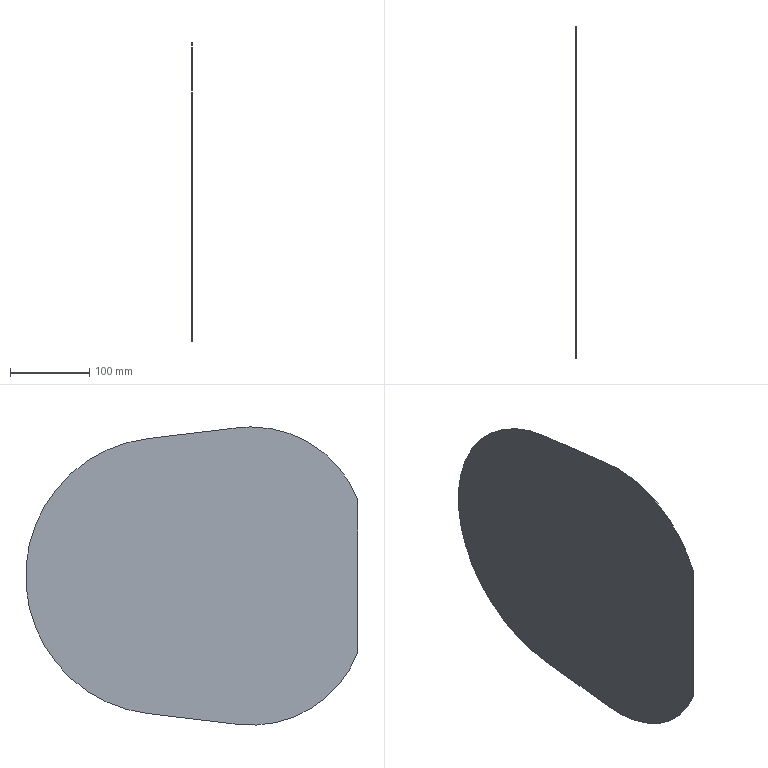Part | STEP file | Input 108 | 1 solid | 9 faces | box 0.5 x 420 x 377 mm | volume 66218 mm3 | plane 5 | cylinder 4 | commonest cylinder face diameters 288 x3 350 x1
STEP:
#1=CARTESIAN_POINT('',(0.,0.,0.));
#2=DIRECTION('',(0.,0.,1.));
#3=DIRECTION('',(1.,0.,0.));
#4=AXIS2_PLACEMENT_3D('',#1,#2,#3);
#5=CARTESIAN_POINT('',(3850.,420.,95.791));
#6=VERTEX_POINT('',#5);
#7=CARTESIAN_POINT('',(3850.,554.4,188.094));
#8=VERTEX_POINT('',#7);
#9=CARTESIAN_POINT('',(3850.,554.4,44.094));
#10=DIRECTION('',(-1.,0.,0.));
#11=DIRECTION('',(0.,0.,-1.));
#12=AXIS2_PLACEMENT_3D('',#9,#10,#11);
#13=CIRCLE('',#12,144.);
#14=CARTESIAN_POINT('',(4469.719,554.4,44.094));
#15=DIRECTION('',(-1.,0.,0.));
#16=DIRECTION('',(0.,0.,1.));
#17=AXIS2_PLACEMENT_3D('',#14,#15,#16);
#18=CYLINDRICAL_SURFACE('',#17,144.);
#19=CARTESIAN_POINT('',(3.142,619.719));
#20=DIRECTION('',(1.,0.));
#21=VECTOR('',#20,1.);
#22=LINE('',#19,#21);
#23=(GEOMETRIC_REPRESENTATION_CONTEXT(2)PARAMETRIC_REPRESENTATION_CONTEXT()REPRESENTATION_CONTEXT('',''));
#24=DEFINITIONAL_REPRESENTATION('',(#22),#23);
#25=PCURVE('',#18,#24);
#26=CARTESIAN_POINT('',(3850.,665.,-0.4063));
#27=DIRECTION('',(1.,0.,0.));
#28=DIRECTION('',(0.,0.,-1.));
#29=AXIS2_PLACEMENT_3D('',#26,#27,#28);
#30=PLANE('',#29);
#31=CARTESIAN_POINT('',(99.5,-110.6));
#32=CARTESIAN_POINT('',(99.5,-360.015));
#33=CARTESIAN_POINT('',(-116.5,-235.308));
#34=CARTESIAN_POINT('',(-332.5,-110.6));
#35=CARTESIAN_POINT('',(-116.5,14.108));
#36=CARTESIAN_POINT('',(99.5,138.815));
#37=CARTESIAN_POINT('',(99.5,-110.6));
#38=(BOUNDED_CURVE()B_SPLINE_CURVE(2,(#31,#32,#33,#34,#35,#36,#37),.UNSPECIFIED.,.T.,.F.)B_SPLINE_CURVE_WITH_KNOTS((1,2,2,2,2,1),(-2.094,0.,2.094,4.189,6.283,8.378),.UNSPECIFIED.)CURVE()GEOMETRIC_REPRESENTATION_ITEM()RATIONAL_B_SPLINE_CURVE((1.,0.5,1.,0.5,1.,0.5,1.))REPRESENTATION_ITEM(''));
#39=(GEOMETRIC_REPRESENTATION_CONTEXT(2)PARAMETRIC_REPRESENTATION_CONTEXT()REPRESENTATION_CONTEXT('',''));
#40=DEFINITIONAL_REPRESENTATION('',(#38),#39);
#41=PCURVE('',#30,#40);
#42=SURFACE_CURVE('',#13,(#25,#41),.PCURVE_S1.);
#43=EDGE_CURVE('',#6,#8,#42,.T.);
#44=ORIENTED_EDGE('',*,*,#43,.T.);
#45=CARTESIAN_POINT('',(3849.5,554.4,188.094));
#46=VERTEX_POINT('',#45);
#47=CARTESIAN_POINT('',(4469.719,554.4,188.094));
#48=DIRECTION('',(-1.,0.,0.));
#49=VECTOR('',#48,1.);
#50=LINE('',#47,#49);
#51=CARTESIAN_POINT('',(6.283,0.));
#52=DIRECTION('',(0.,1.));
#53=VECTOR('',#52,1.);
#54=LINE('',#51,#53);
#55=(GEOMETRIC_REPRESENTATION_CONTEXT(2)PARAMETRIC_REPRESENTATION_CONTEXT()REPRESENTATION_CONTEXT('',''));
#56=DEFINITIONAL_REPRESENTATION('',(#54),#55);
#57=PCURVE('',#18,#56);
#58=CARTESIAN_POINT('',(4469.719,554.4,44.094));
#59=DIRECTION('',(-1.,0.,0.));
#60=DIRECTION('',(0.,0.,1.));
#61=AXIS2_PLACEMENT_3D('',#58,#59,#60);
#62=CYLINDRICAL_SURFACE('',#61,144.);
#63=CARTESIAN_POINT('',(0.,0.));
#64=DIRECTION('',(0.,1.));
#65=VECTOR('',#64,1.);
#66=LINE('',#63,#65);
#67=(GEOMETRIC_REPRESENTATION_CONTEXT(2)PARAMETRIC_REPRESENTATION_CONTEXT()REPRESENTATION_CONTEXT('',''));
#68=DEFINITIONAL_REPRESENTATION('',(#66),#67);
#69=PCURVE('',#62,#68);
#70=SURFACE_CURVE('',#50,(#57,#69),.PCURVE_S1.);
#71=EDGE_CURVE('',#8,#46,#70,.T.);
#72=ORIENTED_EDGE('',*,*,#71,.T.);
#73=CARTESIAN_POINT('',(3849.5,420.,95.791));
#74=VERTEX_POINT('',#73);
#75=CARTESIAN_POINT('',(3849.5,554.4,44.094));
#76=DIRECTION('',(-1.,0.,0.));
#77=DIRECTION('',(0.,0.,1.));
#78=AXIS2_PLACEMENT_3D('',#75,#76,#77);
#79=CIRCLE('',#78,144.);
#80=CARTESIAN_POINT('',(0.,620.219));
#81=DIRECTION('',(1.,0.));
#82=VECTOR('',#81,1.);
#83=LINE('',#80,#82);
#84=(GEOMETRIC_REPRESENTATION_CONTEXT(2)PARAMETRIC_REPRESENTATION_CONTEXT()REPRESENTATION_CONTEXT('',''));
#85=DEFINITIONAL_REPRESENTATION('',(#83),#84);
#86=PCURVE('',#18,#85);
#87=CARTESIAN_POINT('',(3849.5,665.,-0.4063));
#88=DIRECTION('',(-1.,0.,0.));
#89=DIRECTION('',(0.,0.,1.));
#90=AXIS2_PLACEMENT_3D('',#87,#88,#89);
#91=PLANE('',#90);
#92=CARTESIAN_POINT('',(44.5,-110.6));
#93=DIRECTION('',(1.,0.));
#94=AXIS2_PLACEMENT_2D('',#92,#93);
#95=CIRCLE('',#94,144.);
#96=(GEOMETRIC_REPRESENTATION_CONTEXT(2)PARAMETRIC_REPRESENTATION_CONTEXT()REPRESENTATION_CONTEXT('',''));
#97=DEFINITIONAL_REPRESENTATION('',(#95),#96);
#98=PCURVE('',#91,#97);
#99=SURFACE_CURVE('',#79,(#86,#98),.PCURVE_S1.);
#100=EDGE_CURVE('',#74,#46,#99,.T.);
#101=ORIENTED_EDGE('',*,*,#100,.F.);
#102=CARTESIAN_POINT('',(4469.719,420.,95.791));
#103=DIRECTION('',(-1.,0.,0.));
#104=VECTOR('',#103,1.);
#105=LINE('',#102,#104);
#106=CARTESIAN_POINT('',(5.08,0.));
#107=DIRECTION('',(0.,1.));
#108=VECTOR('',#107,1.);
#109=LINE('',#106,#108);
#110=(GEOMETRIC_REPRESENTATION_CONTEXT(2)PARAMETRIC_REPRESENTATION_CONTEXT()REPRESENTATION_CONTEXT('',''));
#111=DEFINITIONAL_REPRESENTATION('',(#109),#110);
#112=PCURVE('',#18,#111);
#113=CARTESIAN_POINT('',(4469.719,420.,-96.604));
#114=DIRECTION('',(0.,-1.,0.));
#115=DIRECTION('',(0.,0.,1.));
#116=AXIS2_PLACEMENT_3D('',#113,#114,#115);
#117=PLANE('',#116);
#118=CARTESIAN_POINT('',(192.395,0.));
#119=DIRECTION('',(0.,1.));
#120=VECTOR('',#119,1.);
#121=LINE('',#118,#120);
#122=(GEOMETRIC_REPRESENTATION_CONTEXT(2)PARAMETRIC_REPRESENTATION_CONTEXT()REPRESENTATION_CONTEXT('',''));
#123=DEFINITIONAL_REPRESENTATION('',(#121),#122);
#124=PCURVE('',#117,#123);
#125=SURFACE_CURVE('',#105,(#112,#124),.PCURVE_S1.);
#126=EDGE_CURVE('',#6,#74,#125,.T.);
#127=ORIENTED_EDGE('',*,*,#126,.F.);
#128=EDGE_LOOP('',(#44,#72,#101,#127));
#129=FACE_BOUND('',#128,.T.);
#130=ADVANCED_FACE('',(#129),#18,.T.);
#131=CARTESIAN_POINT('',(3849.5,685.859,-174.159));
#132=VERTEX_POINT('',#131);
#133=CARTESIAN_POINT('',(3849.5,685.859,173.346));
#134=VERTEX_POINT('',#133);
#135=CARTESIAN_POINT('',(3849.5,665.,-0.4063));
#136=DIRECTION('',(1.,0.,0.));
#137=DIRECTION('',(0.,0.,-1.));
#138=AXIS2_PLACEMENT_3D('',#135,#136,#137);
#139=CIRCLE('',#138,175.);
#140=CARTESIAN_POINT('',(-175.,0.));
#141=CARTESIAN_POINT('',(-175.,303.109));
#142=CARTESIAN_POINT('',(87.5,151.554));
#143=CARTESIAN_POINT('',(350.,0.));
#144=CARTESIAN_POINT('',(87.5,-151.554));
#145=CARTESIAN_POINT('',(-175.,-303.109));
#146=CARTESIAN_POINT('',(-175.,0.));
#147=(BOUNDED_CURVE()B_SPLINE_CURVE(2,(#140,#141,#142,#143,#144,#145,#146),.UNSPECIFIED.,.T.,.F.)B_SPLINE_CURVE_WITH_KNOTS((1,2,2,2,2,1),(-2.094,0.,2.094,4.189,6.283,8.378),.UNSPECIFIED.)CURVE()GEOMETRIC_REPRESENTATION_ITEM()RATIONAL_B_SPLINE_CURVE((1.,0.5,1.,0.5,1.,0.5,1.))REPRESENTATION_ITEM(''));
#148=(GEOMETRIC_REPRESENTATION_CONTEXT(2)PARAMETRIC_REPRESENTATION_CONTEXT()REPRESENTATION_CONTEXT('',''));
#149=DEFINITIONAL_REPRESENTATION('',(#147),#148);
#150=PCURVE('',#91,#149);
#151=CARTESIAN_POINT('',(3850.,665.,-0.4063));
#152=DIRECTION('',(-1.,0.,0.));
#153=DIRECTION('',(0.,0.,1.));
#154=AXIS2_PLACEMENT_3D('',#151,#152,#153);
#155=CYLINDRICAL_SURFACE('',#154,175.);
#156=CARTESIAN_POINT('',(3.142,0.5));
#157=DIRECTION('',(-1.,0.));
#158=VECTOR('',#157,1.);
#159=LINE('',#156,#158);
#160=(GEOMETRIC_REPRESENTATION_CONTEXT(2)PARAMETRIC_REPRESENTATION_CONTEXT()REPRESENTATION_CONTEXT('',''));
#161=DEFINITIONAL_REPRESENTATION('',(#159),#160);
#162=PCURVE('',#155,#161);
#163=SURFACE_CURVE('',#139,(#150,#162),.PCURVE_S1.);
#164=EDGE_CURVE('',#132,#134,#163,.T.);
#165=ORIENTED_EDGE('',*,*,#164,.F.);
#166=CARTESIAN_POINT('',(3849.5,571.564,-187.88));
#167=VERTEX_POINT('',#166);
#168=CARTESIAN_POINT('',(3849.5,685.859,-174.159));
#169=DIRECTION('',(0.,-0.9929,-0.1192));
#170=VECTOR('',#169,1.);
#171=LINE('',#168,#170);
#172=CARTESIAN_POINT('',(-173.752,20.859));
#173=DIRECTION('',(-0.1192,-0.9929));
#174=VECTOR('',#173,1.);
#175=LINE('',#172,#174);
#176=(GEOMETRIC_REPRESENTATION_CONTEXT(2)PARAMETRIC_REPRESENTATION_CONTEXT()REPRESENTATION_CONTEXT('',''));
#177=DEFINITIONAL_REPRESENTATION('',(#175),#176);
#178=PCURVE('',#91,#177);
#179=CARTESIAN_POINT('',(4469.719,685.859,-174.159));
#180=DIRECTION('',(0.,0.1192,-0.9929));
#181=DIRECTION('',(0.,-0.9929,-0.1192));
#182=AXIS2_PLACEMENT_3D('',#179,#180,#181);
#183=PLANE('',#182);
#184=CARTESIAN_POINT('',(0.,620.219));
#185=DIRECTION('',(1.,0.));
#186=VECTOR('',#185,1.);
#187=LINE('',#184,#186);
#188=(GEOMETRIC_REPRESENTATION_CONTEXT(2)PARAMETRIC_REPRESENTATION_CONTEXT()REPRESENTATION_CONTEXT('',''));
#189=DEFINITIONAL_REPRESENTATION('',(#187),#188);
#190=PCURVE('',#183,#189);
#191=SURFACE_CURVE('',#171,(#178,#190),.PCURVE_S1.);
#192=EDGE_CURVE('',#132,#167,#191,.T.);
#193=ORIENTED_EDGE('',*,*,#192,.T.);
#194=CARTESIAN_POINT('',(3849.5,420.,-96.604));
#195=VERTEX_POINT('',#194);
#196=CARTESIAN_POINT('',(3849.5,554.4,-44.906));
#197=DIRECTION('',(-1.,0.,0.));
#198=DIRECTION('',(0.,0.,1.));
#199=AXIS2_PLACEMENT_3D('',#196,#197,#198);
#200=CIRCLE('',#199,144.);
#201=CARTESIAN_POINT('',(-44.5,-110.6));
#202=DIRECTION('',(1.,0.));
#203=AXIS2_PLACEMENT_2D('',#201,#202);
#204=CIRCLE('',#203,144.);
#205=(GEOMETRIC_REPRESENTATION_CONTEXT(2)PARAMETRIC_REPRESENTATION_CONTEXT()REPRESENTATION_CONTEXT('',''));
#206=DEFINITIONAL_REPRESENTATION('',(#204),#205);
#207=PCURVE('',#91,#206);
#208=CARTESIAN_POINT('',(4469.719,554.4,-44.906));
#209=DIRECTION('',(-1.,0.,0.));
#210=DIRECTION('',(0.,0.,1.));
#211=AXIS2_PLACEMENT_3D('',#208,#209,#210);
#212=CYLINDRICAL_SURFACE('',#211,144.);
#213=CARTESIAN_POINT('',(0.,620.219));
#214=DIRECTION('',(1.,0.));
#215=VECTOR('',#214,1.);
#216=LINE('',#213,#215);
#217=(GEOMETRIC_REPRESENTATION_CONTEXT(2)PARAMETRIC_REPRESENTATION_CONTEXT()REPRESENTATION_CONTEXT('',''));
#218=DEFINITIONAL_REPRESENTATION('',(#216),#217);
#219=PCURVE('',#212,#218);
#220=SURFACE_CURVE('',#200,(#207,#219),.PCURVE_S1.);
#221=EDGE_CURVE('',#167,#195,#220,.T.);
#222=ORIENTED_EDGE('',*,*,#221,.T.);
#223=CARTESIAN_POINT('',(3849.5,420.,-96.604));
#224=DIRECTION('',(0.,0.,1.));
#225=VECTOR('',#224,1.);
#226=LINE('',#223,#225);
#227=CARTESIAN_POINT('',(-96.198,-245.));
#228=DIRECTION('',(1.,0.));
#229=VECTOR('',#228,1.);
#230=LINE('',#227,#229);
#231=(GEOMETRIC_REPRESENTATION_CONTEXT(2)PARAMETRIC_REPRESENTATION_CONTEXT()REPRESENTATION_CONTEXT('',''));
#232=DEFINITIONAL_REPRESENTATION('',(#230),#231);
#233=PCURVE('',#91,#232);
#234=CARTESIAN_POINT('',(0.,620.219));
#235=DIRECTION('',(1.,0.));
#236=VECTOR('',#235,1.);
#237=LINE('',#234,#236);
#238=(GEOMETRIC_REPRESENTATION_CONTEXT(2)PARAMETRIC_REPRESENTATION_CONTEXT()REPRESENTATION_CONTEXT('',''));
#239=DEFINITIONAL_REPRESENTATION('',(#237),#238);
#240=PCURVE('',#117,#239);
#241=SURFACE_CURVE('',#226,(#233,#240),.PCURVE_S1.);
#242=EDGE_CURVE('',#195,#74,#241,.T.);
#243=ORIENTED_EDGE('',*,*,#242,.T.);
#244=ORIENTED_EDGE('',*,*,#100,.T.);
#245=CARTESIAN_POINT('',(3849.5,571.564,187.067));
#246=VERTEX_POINT('',#245);
#247=CARTESIAN_POINT('',(3849.5,554.4,44.094));
#248=DIRECTION('',(-1.,0.,0.));
#249=DIRECTION('',(0.,0.,1.));
#250=AXIS2_PLACEMENT_3D('',#247,#248,#249);
#251=CIRCLE('',#250,144.);
#252=CARTESIAN_POINT('',(44.5,-110.6));
#253=DIRECTION('',(1.,0.));
#254=AXIS2_PLACEMENT_2D('',#252,#253);
#255=CIRCLE('',#254,144.);
#256=(GEOMETRIC_REPRESENTATION_CONTEXT(2)PARAMETRIC_REPRESENTATION_CONTEXT()REPRESENTATION_CONTEXT('',''));
#257=DEFINITIONAL_REPRESENTATION('',(#255),#256);
#258=PCURVE('',#91,#257);
#259=CARTESIAN_POINT('',(0.,620.219));
#260=DIRECTION('',(1.,0.));
#261=VECTOR('',#260,1.);
#262=LINE('',#259,#261);
#263=(GEOMETRIC_REPRESENTATION_CONTEXT(2)PARAMETRIC_REPRESENTATION_CONTEXT()REPRESENTATION_CONTEXT('',''));
#264=DEFINITIONAL_REPRESENTATION('',(#262),#263);
#265=PCURVE('',#62,#264);
#266=SURFACE_CURVE('',#251,(#258,#265),.PCURVE_S1.);
#267=EDGE_CURVE('',#46,#246,#266,.T.);
#268=ORIENTED_EDGE('',*,*,#267,.T.);
#269=CARTESIAN_POINT('',(3849.5,571.564,187.067));
#270=DIRECTION('',(0.,0.9929,-0.1192));
#271=VECTOR('',#270,1.);
#272=LINE('',#269,#271);
#273=CARTESIAN_POINT('',(187.473,-93.436));
#274=DIRECTION('',(-0.1192,0.9929));
#275=VECTOR('',#274,1.);
#276=LINE('',#273,#275);
#277=(GEOMETRIC_REPRESENTATION_CONTEXT(2)PARAMETRIC_REPRESENTATION_CONTEXT()REPRESENTATION_CONTEXT('',''));
#278=DEFINITIONAL_REPRESENTATION('',(#276),#277);
#279=PCURVE('',#91,#278);
#280=CARTESIAN_POINT('',(4469.719,571.564,187.067));
#281=DIRECTION('',(0.,0.1192,0.9929));
#282=DIRECTION('',(0.,0.9929,-0.1192));
#283=AXIS2_PLACEMENT_3D('',#280,#281,#282);
#284=PLANE('',#283);
#285=CARTESIAN_POINT('',(0.,620.219));
#286=DIRECTION('',(1.,0.));
#287=VECTOR('',#286,1.);
#288=LINE('',#285,#287);
#289=(GEOMETRIC_REPRESENTATION_CONTEXT(2)PARAMETRIC_REPRESENTATION_CONTEXT()REPRESENTATION_CONTEXT('',''));
#290=DEFINITIONAL_REPRESENTATION('',(#288),#289);
#291=PCURVE('',#284,#290);
#292=SURFACE_CURVE('',#272,(#279,#291),.PCURVE_S1.);
#293=EDGE_CURVE('',#246,#134,#292,.T.);
#294=ORIENTED_EDGE('',*,*,#293,.T.);
#295=EDGE_LOOP('',(#165,#193,#222,#243,#244,#268,#294));
#296=FACE_BOUND('',#295,.T.);
#297=ADVANCED_FACE('',(#296),#91,.T.);
#298=CARTESIAN_POINT('',(3850.,685.859,173.346));
#299=VERTEX_POINT('',#298);
#300=CARTESIAN_POINT('',(3850.,685.859,-174.159));
#301=VERTEX_POINT('',#300);
#302=CARTESIAN_POINT('',(3850.,665.,-0.4063));
#303=DIRECTION('',(-1.,0.,0.));
#304=DIRECTION('',(0.,0.,1.));
#305=AXIS2_PLACEMENT_3D('',#302,#303,#304);
#306=CIRCLE('',#305,175.);
#307=CARTESIAN_POINT('',(-175.,0.));
#308=CARTESIAN_POINT('',(-175.,303.109));
#309=CARTESIAN_POINT('',(87.5,151.554));
#310=CARTESIAN_POINT('',(350.,0.));
#311=CARTESIAN_POINT('',(87.5,-151.554));
#312=CARTESIAN_POINT('',(-175.,-303.109));
#313=CARTESIAN_POINT('',(-175.,0.));
#314=(BOUNDED_CURVE()B_SPLINE_CURVE(2,(#307,#308,#309,#310,#311,#312,#313),.UNSPECIFIED.,.T.,.F.)B_SPLINE_CURVE_WITH_KNOTS((1,2,2,2,2,1),(-2.094,0.,2.094,4.189,6.283,8.378),.UNSPECIFIED.)CURVE()GEOMETRIC_REPRESENTATION_ITEM()RATIONAL_B_SPLINE_CURVE((1.,0.5,1.,0.5,1.,0.5,1.))REPRESENTATION_ITEM(''));
#315=(GEOMETRIC_REPRESENTATION_CONTEXT(2)PARAMETRIC_REPRESENTATION_CONTEXT()REPRESENTATION_CONTEXT('',''));
#316=DEFINITIONAL_REPRESENTATION('',(#314),#315);
#317=PCURVE('',#30,#316);
#318=CARTESIAN_POINT('',(0.,0.));
#319=DIRECTION('',(1.,0.));
#320=VECTOR('',#319,1.);
#321=LINE('',#318,#320);
#322=(GEOMETRIC_REPRESENTATION_CONTEXT(2)PARAMETRIC_REPRESENTATION_CONTEXT()REPRESENTATION_CONTEXT('',''));
#323=DEFINITIONAL_REPRESENTATION('',(#321),#322);
#324=PCURVE('',#155,#323);
#325=SURFACE_CURVE('',#306,(#317,#324),.PCURVE_S1.);
#326=EDGE_CURVE('',#299,#301,#325,.T.);
#327=ORIENTED_EDGE('',*,*,#326,.F.);
#328=CARTESIAN_POINT('',(3850.,571.564,187.067));
#329=VERTEX_POINT('',#328);
#330=CARTESIAN_POINT('',(3850.,571.564,187.067));
#331=DIRECTION('',(0.,0.9929,-0.1192));
#332=VECTOR('',#331,1.);
#333=LINE('',#330,#332);
#334=CARTESIAN_POINT('',(-187.473,-93.436));
#335=DIRECTION('',(0.1192,0.9929));
#336=VECTOR('',#335,1.);
#337=LINE('',#334,#336);
#338=(GEOMETRIC_REPRESENTATION_CONTEXT(2)PARAMETRIC_REPRESENTATION_CONTEXT()REPRESENTATION_CONTEXT('',''));
#339=DEFINITIONAL_REPRESENTATION('',(#337),#338);
#340=PCURVE('',#30,#339);
#341=CARTESIAN_POINT('',(0.,619.719));
#342=DIRECTION('',(1.,0.));
#343=VECTOR('',#342,1.);
#344=LINE('',#341,#343);
#345=(GEOMETRIC_REPRESENTATION_CONTEXT(2)PARAMETRIC_REPRESENTATION_CONTEXT()REPRESENTATION_CONTEXT('',''));
#346=DEFINITIONAL_REPRESENTATION('',(#344),#345);
#347=PCURVE('',#284,#346);
#348=SURFACE_CURVE('',#333,(#340,#347),.PCURVE_S1.);
#349=EDGE_CURVE('',#329,#299,#348,.T.);
#350=ORIENTED_EDGE('',*,*,#349,.F.);
#351=CARTESIAN_POINT('',(3850.,554.4,44.094));
#352=DIRECTION('',(-1.,0.,0.));
#353=DIRECTION('',(0.,0.,-1.));
#354=AXIS2_PLACEMENT_3D('',#351,#352,#353);
#355=CIRCLE('',#354,144.);
#356=CARTESIAN_POINT('',(99.5,-110.6));
#357=CARTESIAN_POINT('',(99.5,-360.015));
#358=CARTESIAN_POINT('',(-116.5,-235.308));
#359=CARTESIAN_POINT('',(-332.5,-110.6));
#360=CARTESIAN_POINT('',(-116.5,14.108));
#361=CARTESIAN_POINT('',(99.5,138.815));
#362=CARTESIAN_POINT('',(99.5,-110.6));
#363=(BOUNDED_CURVE()B_SPLINE_CURVE(2,(#356,#357,#358,#359,#360,#361,#362),.UNSPECIFIED.,.T.,.F.)B_SPLINE_CURVE_WITH_KNOTS((1,2,2,2,2,1),(-2.094,0.,2.094,4.189,6.283,8.378),.UNSPECIFIED.)CURVE()GEOMETRIC_REPRESENTATION_ITEM()RATIONAL_B_SPLINE_CURVE((1.,0.5,1.,0.5,1.,0.5,1.))REPRESENTATION_ITEM(''));
#364=(GEOMETRIC_REPRESENTATION_CONTEXT(2)PARAMETRIC_REPRESENTATION_CONTEXT()REPRESENTATION_CONTEXT('',''));
#365=DEFINITIONAL_REPRESENTATION('',(#363),#364);
#366=PCURVE('',#30,#365);
#367=CARTESIAN_POINT('',(-3.142,619.719));
#368=DIRECTION('',(1.,0.));
#369=VECTOR('',#368,1.);
#370=LINE('',#367,#369);
#371=(GEOMETRIC_REPRESENTATION_CONTEXT(2)PARAMETRIC_REPRESENTATION_CONTEXT()REPRESENTATION_CONTEXT('',''));
#372=DEFINITIONAL_REPRESENTATION('',(#370),#371);
#373=PCURVE('',#62,#372);
#374=SURFACE_CURVE('',#355,(#366,#373),.PCURVE_S1.);
#375=EDGE_CURVE('',#8,#329,#374,.T.);
#376=ORIENTED_EDGE('',*,*,#375,.F.);
#377=ORIENTED_EDGE('',*,*,#43,.F.);
#378=CARTESIAN_POINT('',(3850.,420.,-96.604));
#379=VERTEX_POINT('',#378);
#380=CARTESIAN_POINT('',(3850.,420.,-96.604));
#381=DIRECTION('',(0.,0.,1.));
#382=VECTOR('',#381,1.);
#383=LINE('',#380,#382);
#384=CARTESIAN_POINT('',(96.198,-245.));
#385=DIRECTION('',(-1.,0.));
#386=VECTOR('',#385,1.);
#387=LINE('',#384,#386);
#388=(GEOMETRIC_REPRESENTATION_CONTEXT(2)PARAMETRIC_REPRESENTATION_CONTEXT()REPRESENTATION_CONTEXT('',''));
#389=DEFINITIONAL_REPRESENTATION('',(#387),#388);
#390=PCURVE('',#30,#389);
#391=CARTESIAN_POINT('',(0.,619.719));
#392=DIRECTION('',(1.,0.));
#393=VECTOR('',#392,1.);
#394=LINE('',#391,#393);
#395=(GEOMETRIC_REPRESENTATION_CONTEXT(2)PARAMETRIC_REPRESENTATION_CONTEXT()REPRESENTATION_CONTEXT('',''));
#396=DEFINITIONAL_REPRESENTATION('',(#394),#395);
#397=PCURVE('',#117,#396);
#398=SURFACE_CURVE('',#383,(#390,#397),.PCURVE_S1.);
#399=EDGE_CURVE('',#379,#6,#398,.T.);
#400=ORIENTED_EDGE('',*,*,#399,.F.);
#401=CARTESIAN_POINT('',(3850.,571.564,-187.88));
#402=VERTEX_POINT('',#401);
#403=CARTESIAN_POINT('',(3850.,554.4,-44.906));
#404=DIRECTION('',(-1.,0.,0.));
#405=DIRECTION('',(0.,0.,-1.));
#406=AXIS2_PLACEMENT_3D('',#403,#404,#405);
#407=CIRCLE('',#406,144.);
#408=CARTESIAN_POINT('',(188.5,-110.6));
#409=CARTESIAN_POINT('',(188.5,-360.015));
#410=CARTESIAN_POINT('',(-27.5,-235.308));
#411=CARTESIAN_POINT('',(-243.5,-110.6));
#412=CARTESIAN_POINT('',(-27.5,14.108));
#413=CARTESIAN_POINT('',(188.5,138.815));
#414=CARTESIAN_POINT('',(188.5,-110.6));
#415=(BOUNDED_CURVE()B_SPLINE_CURVE(2,(#408,#409,#410,#411,#412,#413,#414),.UNSPECIFIED.,.T.,.F.)B_SPLINE_CURVE_WITH_KNOTS((1,2,2,2,2,1),(-2.094,0.,2.094,4.189,6.283,8.378),.UNSPECIFIED.)CURVE()GEOMETRIC_REPRESENTATION_ITEM()RATIONAL_B_SPLINE_CURVE((1.,0.5,1.,0.5,1.,0.5,1.))REPRESENTATION_ITEM(''));
#416=(GEOMETRIC_REPRESENTATION_CONTEXT(2)PARAMETRIC_REPRESENTATION_CONTEXT()REPRESENTATION_CONTEXT('',''));
#417=DEFINITIONAL_REPRESENTATION('',(#415),#416);
#418=PCURVE('',#30,#417);
#419=CARTESIAN_POINT('',(-3.142,619.719));
#420=DIRECTION('',(1.,0.));
#421=VECTOR('',#420,1.);
#422=LINE('',#419,#421);
#423=(GEOMETRIC_REPRESENTATION_CONTEXT(2)PARAMETRIC_REPRESENTATION_CONTEXT()REPRESENTATION_CONTEXT('',''));
#424=DEFINITIONAL_REPRESENTATION('',(#422),#423);
#425=PCURVE('',#212,#424);
#426=SURFACE_CURVE('',#407,(#418,#425),.PCURVE_S1.);
#427=EDGE_CURVE('',#402,#379,#426,.T.);
#428=ORIENTED_EDGE('',*,*,#427,.F.);
#429=CARTESIAN_POINT('',(3850.,685.859,-174.159));
#430=DIRECTION('',(0.,-0.9929,-0.1192));
#431=VECTOR('',#430,1.);
#432=LINE('',#429,#431);
#433=CARTESIAN_POINT('',(173.752,20.859));
#434=DIRECTION('',(0.1192,-0.9929));
#435=VECTOR('',#434,1.);
#436=LINE('',#433,#435);
#437=(GEOMETRIC_REPRESENTATION_CONTEXT(2)PARAMETRIC_REPRESENTATION_CONTEXT()REPRESENTATION_CONTEXT('',''));
#438=DEFINITIONAL_REPRESENTATION('',(#436),#437);
#439=PCURVE('',#30,#438);
#440=CARTESIAN_POINT('',(0.,619.719));
#441=DIRECTION('',(1.,0.));
#442=VECTOR('',#441,1.);
#443=LINE('',#440,#442);
#444=(GEOMETRIC_REPRESENTATION_CONTEXT(2)PARAMETRIC_REPRESENTATION_CONTEXT()REPRESENTATION_CONTEXT('',''));
#445=DEFINITIONAL_REPRESENTATION('',(#443),#444);
#446=PCURVE('',#183,#445);
#447=SURFACE_CURVE('',#432,(#439,#446),.PCURVE_S1.);
#448=EDGE_CURVE('',#301,#402,#447,.T.);
#449=ORIENTED_EDGE('',*,*,#448,.F.);
#450=EDGE_LOOP('',(#327,#350,#376,#377,#400,#428,#449));
#451=FACE_BOUND('',#450,.T.);
#452=ADVANCED_FACE('',(#451),#30,.T.);
#453=CARTESIAN_POINT('',(4469.719,685.859,-174.159));
#454=DIRECTION('',(-1.,0.,0.));
#455=VECTOR('',#454,1.);
#456=LINE('',#453,#455);
#457=CARTESIAN_POINT('',(3.022,-619.719));
#458=DIRECTION('',(0.,1.));
#459=VECTOR('',#458,1.);
#460=LINE('',#457,#459);
#461=(GEOMETRIC_REPRESENTATION_CONTEXT(2)PARAMETRIC_REPRESENTATION_CONTEXT()REPRESENTATION_CONTEXT('',''));
#462=DEFINITIONAL_REPRESENTATION('',(#460),#461);
#463=PCURVE('',#155,#462);
#464=CARTESIAN_POINT('',(0.,0.));
#465=DIRECTION('',(0.,1.));
#466=VECTOR('',#465,1.);
#467=LINE('',#464,#466);
#468=(GEOMETRIC_REPRESENTATION_CONTEXT(2)PARAMETRIC_REPRESENTATION_CONTEXT()REPRESENTATION_CONTEXT('',''));
#469=DEFINITIONAL_REPRESENTATION('',(#467),#468);
#470=PCURVE('',#183,#469);
#471=SURFACE_CURVE('',#456,(#463,#470),.PCURVE_S1.);
#472=EDGE_CURVE('',#301,#132,#471,.T.);
#473=ORIENTED_EDGE('',*,*,#472,.T.);
#474=ORIENTED_EDGE('',*,*,#164,.T.);
#475=CARTESIAN_POINT('',(4469.719,685.859,173.346));
#476=DIRECTION('',(-1.,0.,0.));
#477=VECTOR('',#476,1.);
#478=LINE('',#475,#477);
#479=CARTESIAN_POINT('',(0.1195,-619.719));
#480=DIRECTION('',(0.,1.));
#481=VECTOR('',#480,1.);
#482=LINE('',#479,#481);
#483=(GEOMETRIC_REPRESENTATION_CONTEXT(2)PARAMETRIC_REPRESENTATION_CONTEXT()REPRESENTATION_CONTEXT('',''));
#484=DEFINITIONAL_REPRESENTATION('',(#482),#483);
#485=PCURVE('',#155,#484);
#486=CARTESIAN_POINT('',(115.116,0.));
#487=DIRECTION('',(0.,1.));
#488=VECTOR('',#487,1.);
#489=LINE('',#486,#488);
#490=(GEOMETRIC_REPRESENTATION_CONTEXT(2)PARAMETRIC_REPRESENTATION_CONTEXT()REPRESENTATION_CONTEXT('',''));
#491=DEFINITIONAL_REPRESENTATION('',(#489),#490);
#492=PCURVE('',#284,#491);
#493=SURFACE_CURVE('',#478,(#485,#492),.PCURVE_S1.);
#494=EDGE_CURVE('',#299,#134,#493,.T.);
#495=ORIENTED_EDGE('',*,*,#494,.F.);
#496=ORIENTED_EDGE('',*,*,#326,.T.);
#497=EDGE_LOOP('',(#473,#474,#495,#496));
#498=FACE_BOUND('',#497,.T.);
#499=ADVANCED_FACE('',(#498),#155,.T.);
#500=ORIENTED_EDGE('',*,*,#192,.F.);
#501=ORIENTED_EDGE('',*,*,#472,.F.);
#502=ORIENTED_EDGE('',*,*,#448,.T.);
#503=CARTESIAN_POINT('',(4469.719,571.564,-187.88));
#504=DIRECTION('',(-1.,0.,0.));
#505=VECTOR('',#504,1.);
#506=LINE('',#503,#505);
#507=CARTESIAN_POINT('',(115.116,0.));
#508=DIRECTION('',(0.,1.));
#509=VECTOR('',#508,1.);
#510=LINE('',#507,#509);
#511=(GEOMETRIC_REPRESENTATION_CONTEXT(2)PARAMETRIC_REPRESENTATION_CONTEXT()REPRESENTATION_CONTEXT('',''));
#512=DEFINITIONAL_REPRESENTATION('',(#510),#511);
#513=PCURVE('',#183,#512);
#514=CARTESIAN_POINT('',(3.022,0.));
#515=DIRECTION('',(0.,1.));
#516=VECTOR('',#515,1.);
#517=LINE('',#514,#516);
#518=(GEOMETRIC_REPRESENTATION_CONTEXT(2)PARAMETRIC_REPRESENTATION_CONTEXT()REPRESENTATION_CONTEXT('',''));
#519=DEFINITIONAL_REPRESENTATION('',(#517),#518);
#520=PCURVE('',#212,#519);
#521=SURFACE_CURVE('',#506,(#513,#520),.PCURVE_S1.);
#522=EDGE_CURVE('',#402,#167,#521,.T.);
#523=ORIENTED_EDGE('',*,*,#522,.T.);
#524=EDGE_LOOP('',(#500,#501,#502,#523));
#525=FACE_BOUND('',#524,.T.);
#526=ADVANCED_FACE('',(#525),#183,.T.);
#527=ORIENTED_EDGE('',*,*,#221,.F.);
#528=ORIENTED_EDGE('',*,*,#522,.F.);
#529=ORIENTED_EDGE('',*,*,#427,.T.);
#530=CARTESIAN_POINT('',(4469.719,420.,-96.604));
#531=DIRECTION('',(-1.,0.,0.));
#532=VECTOR('',#531,1.);
#533=LINE('',#530,#532);
#534=CARTESIAN_POINT('',(4.345,0.));
#535=DIRECTION('',(0.,1.));
#536=VECTOR('',#535,1.);
#537=LINE('',#534,#536);
#538=(GEOMETRIC_REPRESENTATION_CONTEXT(2)PARAMETRIC_REPRESENTATION_CONTEXT()REPRESENTATION_CONTEXT('',''));
#539=DEFINITIONAL_REPRESENTATION('',(#537),#538);
#540=PCURVE('',#212,#539);
#541=CARTESIAN_POINT('',(0.,0.));
#542=DIRECTION('',(0.,1.));
#543=VECTOR('',#542,1.);
#544=LINE('',#541,#543);
#545=(GEOMETRIC_REPRESENTATION_CONTEXT(2)PARAMETRIC_REPRESENTATION_CONTEXT()REPRESENTATION_CONTEXT('',''));
#546=DEFINITIONAL_REPRESENTATION('',(#544),#545);
#547=PCURVE('',#117,#546);
#548=SURFACE_CURVE('',#533,(#540,#547),.PCURVE_S1.);
#549=EDGE_CURVE('',#379,#195,#548,.T.);
#550=ORIENTED_EDGE('',*,*,#549,.T.);
#551=EDGE_LOOP('',(#527,#528,#529,#550));
#552=FACE_BOUND('',#551,.T.);
#553=ADVANCED_FACE('',(#552),#212,.T.);
#554=ORIENTED_EDGE('',*,*,#242,.F.);
#555=ORIENTED_EDGE('',*,*,#549,.F.);
#556=ORIENTED_EDGE('',*,*,#399,.T.);
#557=ORIENTED_EDGE('',*,*,#126,.T.);
#558=EDGE_LOOP('',(#554,#555,#556,#557));
#559=FACE_BOUND('',#558,.T.);
#560=ADVANCED_FACE('',(#559),#117,.T.);
#561=ORIENTED_EDGE('',*,*,#71,.F.);
#562=ORIENTED_EDGE('',*,*,#375,.T.);
#563=CARTESIAN_POINT('',(4469.719,571.564,187.067));
#564=DIRECTION('',(-1.,0.,0.));
#565=VECTOR('',#564,1.);
#566=LINE('',#563,#565);
#567=CARTESIAN_POINT('',(0.1195,0.));
#568=DIRECTION('',(0.,1.));
#569=VECTOR('',#568,1.);
#570=LINE('',#567,#569);
#571=(GEOMETRIC_REPRESENTATION_CONTEXT(2)PARAMETRIC_REPRESENTATION_CONTEXT()REPRESENTATION_CONTEXT('',''));
#572=DEFINITIONAL_REPRESENTATION('',(#570),#571);
#573=PCURVE('',#62,#572);
#574=CARTESIAN_POINT('',(0.,0.));
#575=DIRECTION('',(0.,1.));
#576=VECTOR('',#575,1.);
#577=LINE('',#574,#576);
#578=(GEOMETRIC_REPRESENTATION_CONTEXT(2)PARAMETRIC_REPRESENTATION_CONTEXT()REPRESENTATION_CONTEXT('',''));
#579=DEFINITIONAL_REPRESENTATION('',(#577),#578);
#580=PCURVE('',#284,#579);
#581=SURFACE_CURVE('',#566,(#573,#580),.PCURVE_S1.);
#582=EDGE_CURVE('',#329,#246,#581,.T.);
#583=ORIENTED_EDGE('',*,*,#582,.T.);
#584=ORIENTED_EDGE('',*,*,#267,.F.);
#585=EDGE_LOOP('',(#561,#562,#583,#584));
#586=FACE_BOUND('',#585,.T.);
#587=ADVANCED_FACE('',(#586),#62,.T.);
#588=ORIENTED_EDGE('',*,*,#293,.F.);
#589=ORIENTED_EDGE('',*,*,#582,.F.);
#590=ORIENTED_EDGE('',*,*,#349,.T.);
#591=ORIENTED_EDGE('',*,*,#494,.T.);
#592=EDGE_LOOP('',(#588,#589,#590,#591));
#593=FACE_BOUND('',#592,.T.);
#594=ADVANCED_FACE('',(#593),#284,.T.);
#595=CLOSED_SHELL('',(#130,#297,#452,#499,#526,#553,#560,#587,#594));
#596=MANIFOLD_SOLID_BREP('',#595);
#597=(LENGTH_UNIT()NAMED_UNIT(*)SI_UNIT(.MILLI.,.METRE.));
#598=UNCERTAINTY_MEASURE_WITH_UNIT(LENGTH_MEASURE(0.0000001),#597,'','');
#599=(NAMED_UNIT(*)PLANE_ANGLE_UNIT()SI_UNIT($,.RADIAN.));
#600=(NAMED_UNIT(*)SI_UNIT($,.STERADIAN.)SOLID_ANGLE_UNIT());
#601=(GEOMETRIC_REPRESENTATION_CONTEXT(3)GLOBAL_UNCERTAINTY_ASSIGNED_CONTEXT((#598))GLOBAL_UNIT_ASSIGNED_CONTEXT((#597,#599,#600))REPRESENTATION_CONTEXT('',''));
#602=ADVANCED_BREP_SHAPE_REPRESENTATION('',(#4,#596),#601);